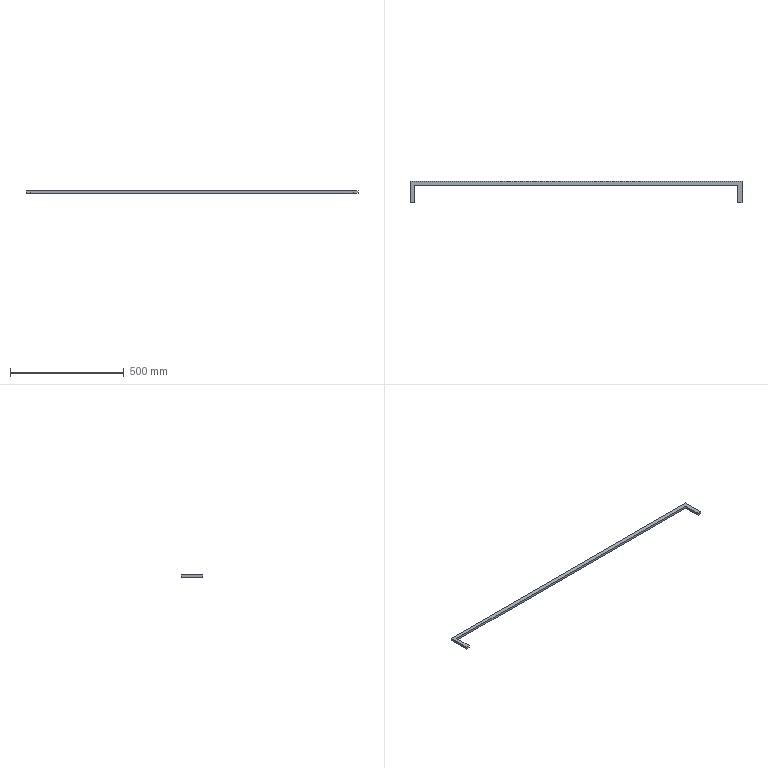Part | STEP file | 1 solid | 10 faces | box 1458 x 94 x 10 mm | volume 289800 mm3 | plane 10
STEP:
#1=CARTESIAN_POINT('',(0.,0.,0.));
#2=DIRECTION('',(0.,0.,1.));
#3=DIRECTION('',(1.,0.,0.));
#4=AXIS2_PLACEMENT_3D('',#1,#2,#3);
#5=CARTESIAN_POINT('',(-18.,0.,0.));
#6=VERTEX_POINT('',#5);
#7=CARTESIAN_POINT('',(-18.,94.,0.));
#8=VERTEX_POINT('',#7);
#9=CARTESIAN_POINT('',(-18.,0.,0.));
#10=DIRECTION('',(0.,1.,0.));
#11=VECTOR('',#10,1.);
#12=LINE('',#9,#11);
#13=CARTESIAN_POINT('',(1422.,0.,0.));
#14=DIRECTION('',(0.,0.,-1.));
#15=DIRECTION('',(-1.,0.,0.));
#16=AXIS2_PLACEMENT_3D('',#13,#14,#15);
#17=PLANE('',#16);
#18=CARTESIAN_POINT('',(1440.,0.));
#19=DIRECTION('',(0.,1.));
#20=VECTOR('',#19,1.);
#21=LINE('',#18,#20);
#22=(GEOMETRIC_REPRESENTATION_CONTEXT(2)PARAMETRIC_REPRESENTATION_CONTEXT()REPRESENTATION_CONTEXT('',''));
#23=DEFINITIONAL_REPRESENTATION('',(#21),#22);
#24=PCURVE('',#17,#23);
#25=CARTESIAN_POINT('',(-18.,0.,10.));
#26=DIRECTION('',(-1.,0.,0.));
#27=DIRECTION('',(0.,0.,1.));
#28=AXIS2_PLACEMENT_3D('',#25,#26,#27);
#29=PLANE('',#28);
#30=CARTESIAN_POINT('',(-10.,0.));
#31=DIRECTION('',(0.,1.));
#32=VECTOR('',#31,1.);
#33=LINE('',#30,#32);
#34=(GEOMETRIC_REPRESENTATION_CONTEXT(2)PARAMETRIC_REPRESENTATION_CONTEXT()REPRESENTATION_CONTEXT('',''));
#35=DEFINITIONAL_REPRESENTATION('',(#33),#34);
#36=PCURVE('',#29,#35);
#37=SURFACE_CURVE('',#12,(#24,#36),.PCURVE_S1.);
#38=EDGE_CURVE('',#6,#8,#37,.T.);
#39=ORIENTED_EDGE('',*,*,#38,.T.);
#40=CARTESIAN_POINT('',(1440.,94.,0.));
#41=VERTEX_POINT('',#40);
#42=CARTESIAN_POINT('',(1422.,94.,0.));
#43=DIRECTION('',(1.,0.,0.));
#44=VECTOR('',#43,1.);
#45=LINE('',#42,#44);
#46=CARTESIAN_POINT('',(0.,94.));
#47=DIRECTION('',(-1.,0.));
#48=VECTOR('',#47,1.);
#49=LINE('',#46,#48);
#50=(GEOMETRIC_REPRESENTATION_CONTEXT(2)PARAMETRIC_REPRESENTATION_CONTEXT()REPRESENTATION_CONTEXT('',''));
#51=DEFINITIONAL_REPRESENTATION('',(#49),#50);
#52=PCURVE('',#17,#51);
#53=CARTESIAN_POINT('',(0.,94.,10.));
#54=DIRECTION('',(0.,1.,0.));
#55=DIRECTION('',(0.,0.,1.));
#56=AXIS2_PLACEMENT_3D('',#53,#54,#55);
#57=PLANE('',#56);
#58=CARTESIAN_POINT('',(-10.,1422.));
#59=DIRECTION('',(0.,1.));
#60=VECTOR('',#59,1.);
#61=LINE('',#58,#60);
#62=(GEOMETRIC_REPRESENTATION_CONTEXT(2)PARAMETRIC_REPRESENTATION_CONTEXT()REPRESENTATION_CONTEXT('',''));
#63=DEFINITIONAL_REPRESENTATION('',(#61),#62);
#64=PCURVE('',#57,#63);
#65=SURFACE_CURVE('',#45,(#52,#64),.PCURVE_S1.);
#66=EDGE_CURVE('',#8,#41,#65,.T.);
#67=ORIENTED_EDGE('',*,*,#66,.T.);
#68=CARTESIAN_POINT('',(1440.,0.,0.));
#69=VERTEX_POINT('',#68);
#70=CARTESIAN_POINT('',(1440.,0.,0.));
#71=DIRECTION('',(0.,-1.,0.));
#72=VECTOR('',#71,1.);
#73=LINE('',#70,#72);
#74=CARTESIAN_POINT('',(-18.,0.));
#75=DIRECTION('',(0.,-1.));
#76=VECTOR('',#75,1.);
#77=LINE('',#74,#76);
#78=(GEOMETRIC_REPRESENTATION_CONTEXT(2)PARAMETRIC_REPRESENTATION_CONTEXT()REPRESENTATION_CONTEXT('',''));
#79=DEFINITIONAL_REPRESENTATION('',(#77),#78);
#80=PCURVE('',#17,#79);
#81=CARTESIAN_POINT('',(1440.,76.,10.));
#82=DIRECTION('',(1.,0.,0.));
#83=DIRECTION('',(0.,0.,-1.));
#84=AXIS2_PLACEMENT_3D('',#81,#82,#83);
#85=PLANE('',#84);
#86=CARTESIAN_POINT('',(10.,-76.));
#87=DIRECTION('',(0.,-1.));
#88=VECTOR('',#87,1.);
#89=LINE('',#86,#88);
#90=(GEOMETRIC_REPRESENTATION_CONTEXT(2)PARAMETRIC_REPRESENTATION_CONTEXT()REPRESENTATION_CONTEXT('',''));
#91=DEFINITIONAL_REPRESENTATION('',(#89),#90);
#92=PCURVE('',#85,#91);
#93=SURFACE_CURVE('',#73,(#80,#92),.PCURVE_S1.);
#94=EDGE_CURVE('',#41,#69,#93,.T.);
#95=ORIENTED_EDGE('',*,*,#94,.T.);
#96=CARTESIAN_POINT('',(1422.,0.,0.));
#97=VERTEX_POINT('',#96);
#98=CARTESIAN_POINT('',(1422.,0.,0.));
#99=DIRECTION('',(-1.,0.,0.));
#100=VECTOR('',#99,1.);
#101=LINE('',#98,#100);
#102=CARTESIAN_POINT('',(0.,0.));
#103=DIRECTION('',(1.,0.));
#104=VECTOR('',#103,1.);
#105=LINE('',#102,#104);
#106=(GEOMETRIC_REPRESENTATION_CONTEXT(2)PARAMETRIC_REPRESENTATION_CONTEXT()REPRESENTATION_CONTEXT('',''));
#107=DEFINITIONAL_REPRESENTATION('',(#105),#106);
#108=PCURVE('',#17,#107);
#109=CARTESIAN_POINT('',(1440.,0.,10.));
#110=DIRECTION('',(0.,-1.,0.));
#111=DIRECTION('',(0.,0.,-1.));
#112=AXIS2_PLACEMENT_3D('',#109,#110,#111);
#113=PLANE('',#112);
#114=CARTESIAN_POINT('',(10.,-18.));
#115=DIRECTION('',(0.,-1.));
#116=VECTOR('',#115,1.);
#117=LINE('',#114,#116);
#118=(GEOMETRIC_REPRESENTATION_CONTEXT(2)PARAMETRIC_REPRESENTATION_CONTEXT()REPRESENTATION_CONTEXT('',''));
#119=DEFINITIONAL_REPRESENTATION('',(#117),#118);
#120=PCURVE('',#113,#119);
#121=SURFACE_CURVE('',#101,(#108,#120),.PCURVE_S1.);
#122=EDGE_CURVE('',#69,#97,#121,.T.);
#123=ORIENTED_EDGE('',*,*,#122,.T.);
#124=CARTESIAN_POINT('',(1422.,76.,0.));
#125=VERTEX_POINT('',#124);
#126=CARTESIAN_POINT('',(1422.,0.,0.));
#127=DIRECTION('',(0.,1.,0.));
#128=VECTOR('',#127,1.);
#129=LINE('',#126,#128);
#130=CARTESIAN_POINT('',(0.,0.));
#131=DIRECTION('',(0.,1.));
#132=VECTOR('',#131,1.);
#133=LINE('',#130,#132);
#134=(GEOMETRIC_REPRESENTATION_CONTEXT(2)PARAMETRIC_REPRESENTATION_CONTEXT()REPRESENTATION_CONTEXT('',''));
#135=DEFINITIONAL_REPRESENTATION('',(#133),#134);
#136=PCURVE('',#17,#135);
#137=CARTESIAN_POINT('',(1422.,76.,10.));
#138=DIRECTION('',(1.,0.,0.));
#139=DIRECTION('',(0.,0.,-1.));
#140=AXIS2_PLACEMENT_3D('',#137,#138,#139);
#141=PLANE('',#140);
#142=CARTESIAN_POINT('',(10.,-76.));
#143=DIRECTION('',(0.,1.));
#144=VECTOR('',#143,1.);
#145=LINE('',#142,#144);
#146=(GEOMETRIC_REPRESENTATION_CONTEXT(2)PARAMETRIC_REPRESENTATION_CONTEXT()REPRESENTATION_CONTEXT('',''));
#147=DEFINITIONAL_REPRESENTATION('',(#145),#146);
#148=PCURVE('',#141,#147);
#149=SURFACE_CURVE('',#129,(#136,#148),.PCURVE_S1.);
#150=EDGE_CURVE('',#97,#125,#149,.T.);
#151=ORIENTED_EDGE('',*,*,#150,.T.);
#152=CARTESIAN_POINT('',(0.,76.,0.));
#153=VERTEX_POINT('',#152);
#154=CARTESIAN_POINT('',(1422.,76.,0.));
#155=DIRECTION('',(-1.,0.,0.));
#156=VECTOR('',#155,1.);
#157=LINE('',#154,#156);
#158=CARTESIAN_POINT('',(0.,76.));
#159=DIRECTION('',(1.,0.));
#160=VECTOR('',#159,1.);
#161=LINE('',#158,#160);
#162=(GEOMETRIC_REPRESENTATION_CONTEXT(2)PARAMETRIC_REPRESENTATION_CONTEXT()REPRESENTATION_CONTEXT('',''));
#163=DEFINITIONAL_REPRESENTATION('',(#161),#162);
#164=PCURVE('',#17,#163);
#165=CARTESIAN_POINT('',(0.,76.,10.));
#166=DIRECTION('',(0.,1.,0.));
#167=DIRECTION('',(0.,0.,1.));
#168=AXIS2_PLACEMENT_3D('',#165,#166,#167);
#169=PLANE('',#168);
#170=CARTESIAN_POINT('',(-10.,1422.));
#171=DIRECTION('',(0.,-1.));
#172=VECTOR('',#171,1.);
#173=LINE('',#170,#172);
#174=(GEOMETRIC_REPRESENTATION_CONTEXT(2)PARAMETRIC_REPRESENTATION_CONTEXT()REPRESENTATION_CONTEXT('',''));
#175=DEFINITIONAL_REPRESENTATION('',(#173),#174);
#176=PCURVE('',#169,#175);
#177=SURFACE_CURVE('',#157,(#164,#176),.PCURVE_S1.);
#178=EDGE_CURVE('',#125,#153,#177,.T.);
#179=ORIENTED_EDGE('',*,*,#178,.T.);
#180=CARTESIAN_POINT('',(0.,0.,0.));
#181=VERTEX_POINT('',#180);
#182=CARTESIAN_POINT('',(0.,0.,0.));
#183=DIRECTION('',(0.,-1.,0.));
#184=VECTOR('',#183,1.);
#185=LINE('',#182,#184);
#186=CARTESIAN_POINT('',(1422.,0.));
#187=DIRECTION('',(0.,-1.));
#188=VECTOR('',#187,1.);
#189=LINE('',#186,#188);
#190=(GEOMETRIC_REPRESENTATION_CONTEXT(2)PARAMETRIC_REPRESENTATION_CONTEXT()REPRESENTATION_CONTEXT('',''));
#191=DEFINITIONAL_REPRESENTATION('',(#189),#190);
#192=PCURVE('',#17,#191);
#193=CARTESIAN_POINT('',(0.,0.,10.));
#194=DIRECTION('',(-1.,0.,0.));
#195=DIRECTION('',(0.,0.,1.));
#196=AXIS2_PLACEMENT_3D('',#193,#194,#195);
#197=PLANE('',#196);
#198=CARTESIAN_POINT('',(-10.,0.));
#199=DIRECTION('',(0.,-1.));
#200=VECTOR('',#199,1.);
#201=LINE('',#198,#200);
#202=(GEOMETRIC_REPRESENTATION_CONTEXT(2)PARAMETRIC_REPRESENTATION_CONTEXT()REPRESENTATION_CONTEXT('',''));
#203=DEFINITIONAL_REPRESENTATION('',(#201),#202);
#204=PCURVE('',#197,#203);
#205=SURFACE_CURVE('',#185,(#192,#204),.PCURVE_S1.);
#206=EDGE_CURVE('',#153,#181,#205,.T.);
#207=ORIENTED_EDGE('',*,*,#206,.T.);
#208=CARTESIAN_POINT('',(1422.,0.,0.));
#209=DIRECTION('',(-1.,0.,0.));
#210=VECTOR('',#209,1.);
#211=LINE('',#208,#210);
#212=CARTESIAN_POINT('',(0.,0.));
#213=DIRECTION('',(1.,0.));
#214=VECTOR('',#213,1.);
#215=LINE('',#212,#214);
#216=(GEOMETRIC_REPRESENTATION_CONTEXT(2)PARAMETRIC_REPRESENTATION_CONTEXT()REPRESENTATION_CONTEXT('',''));
#217=DEFINITIONAL_REPRESENTATION('',(#215),#216);
#218=PCURVE('',#17,#217);
#219=CARTESIAN_POINT('',(0.,0.,10.));
#220=DIRECTION('',(0.,-1.,0.));
#221=DIRECTION('',(0.,0.,-1.));
#222=AXIS2_PLACEMENT_3D('',#219,#220,#221);
#223=PLANE('',#222);
#224=CARTESIAN_POINT('',(10.,1422.));
#225=DIRECTION('',(0.,-1.));
#226=VECTOR('',#225,1.);
#227=LINE('',#224,#226);
#228=(GEOMETRIC_REPRESENTATION_CONTEXT(2)PARAMETRIC_REPRESENTATION_CONTEXT()REPRESENTATION_CONTEXT('',''));
#229=DEFINITIONAL_REPRESENTATION('',(#227),#228);
#230=PCURVE('',#223,#229);
#231=SURFACE_CURVE('',#211,(#218,#230),.PCURVE_S1.);
#232=EDGE_CURVE('',#181,#6,#231,.T.);
#233=ORIENTED_EDGE('',*,*,#232,.T.);
#234=EDGE_LOOP('',(#39,#67,#95,#123,#151,#179,#207,#233));
#235=FACE_BOUND('',#234,.T.);
#236=ADVANCED_FACE('',(#235),#17,.T.);
#237=ORIENTED_EDGE('',*,*,#66,.F.);
#238=CARTESIAN_POINT('',(-18.,94.,10.));
#239=VERTEX_POINT('',#238);
#240=CARTESIAN_POINT('',(-18.,94.,10.));
#241=DIRECTION('',(0.,0.,1.));
#242=VECTOR('',#241,1.);
#243=LINE('',#240,#242);
#244=CARTESIAN_POINT('',(0.,-18.));
#245=DIRECTION('',(1.,0.));
#246=VECTOR('',#245,1.);
#247=LINE('',#244,#246);
#248=(GEOMETRIC_REPRESENTATION_CONTEXT(2)PARAMETRIC_REPRESENTATION_CONTEXT()REPRESENTATION_CONTEXT('',''));
#249=DEFINITIONAL_REPRESENTATION('',(#247),#248);
#250=PCURVE('',#57,#249);
#251=CARTESIAN_POINT('',(0.,94.));
#252=DIRECTION('',(1.,0.));
#253=VECTOR('',#252,1.);
#254=LINE('',#251,#253);
#255=(GEOMETRIC_REPRESENTATION_CONTEXT(2)PARAMETRIC_REPRESENTATION_CONTEXT()REPRESENTATION_CONTEXT('',''));
#256=DEFINITIONAL_REPRESENTATION('',(#254),#255);
#257=PCURVE('',#29,#256);
#258=SURFACE_CURVE('',#243,(#250,#257),.PCURVE_S1.);
#259=EDGE_CURVE('',#8,#239,#258,.T.);
#260=ORIENTED_EDGE('',*,*,#259,.T.);
#261=CARTESIAN_POINT('',(1440.,94.,10.));
#262=VERTEX_POINT('',#261);
#263=CARTESIAN_POINT('',(0.,94.,10.));
#264=DIRECTION('',(1.,0.,0.));
#265=VECTOR('',#264,1.);
#266=LINE('',#263,#265);
#267=CARTESIAN_POINT('',(0.,0.));
#268=DIRECTION('',(0.,1.));
#269=VECTOR('',#268,1.);
#270=LINE('',#267,#269);
#271=(GEOMETRIC_REPRESENTATION_CONTEXT(2)PARAMETRIC_REPRESENTATION_CONTEXT()REPRESENTATION_CONTEXT('',''));
#272=DEFINITIONAL_REPRESENTATION('',(#270),#271);
#273=PCURVE('',#57,#272);
#274=CARTESIAN_POINT('',(1422.,0.,10.));
#275=DIRECTION('',(0.,0.,-1.));
#276=DIRECTION('',(-1.,0.,0.));
#277=AXIS2_PLACEMENT_3D('',#274,#275,#276);
#278=PLANE('',#277);
#279=CARTESIAN_POINT('',(1422.,94.));
#280=DIRECTION('',(-1.,0.));
#281=VECTOR('',#280,1.);
#282=LINE('',#279,#281);
#283=(GEOMETRIC_REPRESENTATION_CONTEXT(2)PARAMETRIC_REPRESENTATION_CONTEXT()REPRESENTATION_CONTEXT('',''));
#284=DEFINITIONAL_REPRESENTATION('',(#282),#283);
#285=PCURVE('',#278,#284);
#286=SURFACE_CURVE('',#266,(#273,#285),.PCURVE_S1.);
#287=EDGE_CURVE('',#239,#262,#286,.T.);
#288=ORIENTED_EDGE('',*,*,#287,.T.);
#289=CARTESIAN_POINT('',(1440.,94.,10.));
#290=DIRECTION('',(0.,0.,-1.));
#291=VECTOR('',#290,1.);
#292=LINE('',#289,#291);
#293=CARTESIAN_POINT('',(0.,1440.));
#294=DIRECTION('',(-1.,0.));
#295=VECTOR('',#294,1.);
#296=LINE('',#293,#295);
#297=(GEOMETRIC_REPRESENTATION_CONTEXT(2)PARAMETRIC_REPRESENTATION_CONTEXT()REPRESENTATION_CONTEXT('',''));
#298=DEFINITIONAL_REPRESENTATION('',(#296),#297);
#299=PCURVE('',#57,#298);
#300=CARTESIAN_POINT('',(0.,18.));
#301=DIRECTION('',(1.,0.));
#302=VECTOR('',#301,1.);
#303=LINE('',#300,#302);
#304=(GEOMETRIC_REPRESENTATION_CONTEXT(2)PARAMETRIC_REPRESENTATION_CONTEXT()REPRESENTATION_CONTEXT('',''));
#305=DEFINITIONAL_REPRESENTATION('',(#303),#304);
#306=PCURVE('',#85,#305);
#307=SURFACE_CURVE('',#292,(#299,#306),.PCURVE_S1.);
#308=EDGE_CURVE('',#262,#41,#307,.T.);
#309=ORIENTED_EDGE('',*,*,#308,.T.);
#310=EDGE_LOOP('',(#237,#260,#288,#309));
#311=FACE_BOUND('',#310,.T.);
#312=ADVANCED_FACE('',(#311),#57,.T.);
#313=ORIENTED_EDGE('',*,*,#38,.F.);
#314=CARTESIAN_POINT('',(-18.,0.,10.));
#315=VERTEX_POINT('',#314);
#316=CARTESIAN_POINT('',(-18.,0.,10.));
#317=DIRECTION('',(0.,0.,1.));
#318=VECTOR('',#317,1.);
#319=LINE('',#316,#318);
#320=CARTESIAN_POINT('',(0.,0.));
#321=DIRECTION('',(1.,0.));
#322=VECTOR('',#321,1.);
#323=LINE('',#320,#322);
#324=(GEOMETRIC_REPRESENTATION_CONTEXT(2)PARAMETRIC_REPRESENTATION_CONTEXT()REPRESENTATION_CONTEXT('',''));
#325=DEFINITIONAL_REPRESENTATION('',(#323),#324);
#326=PCURVE('',#29,#325);
#327=CARTESIAN_POINT('',(0.,-18.));
#328=DIRECTION('',(-1.,0.));
#329=VECTOR('',#328,1.);
#330=LINE('',#327,#329);
#331=(GEOMETRIC_REPRESENTATION_CONTEXT(2)PARAMETRIC_REPRESENTATION_CONTEXT()REPRESENTATION_CONTEXT('',''));
#332=DEFINITIONAL_REPRESENTATION('',(#330),#331);
#333=PCURVE('',#223,#332);
#334=SURFACE_CURVE('',#319,(#326,#333),.PCURVE_S1.);
#335=EDGE_CURVE('',#6,#315,#334,.T.);
#336=ORIENTED_EDGE('',*,*,#335,.T.);
#337=CARTESIAN_POINT('',(-18.,0.,10.));
#338=DIRECTION('',(0.,1.,0.));
#339=VECTOR('',#338,1.);
#340=LINE('',#337,#339);
#341=CARTESIAN_POINT('',(0.,0.));
#342=DIRECTION('',(0.,1.));
#343=VECTOR('',#342,1.);
#344=LINE('',#341,#343);
#345=(GEOMETRIC_REPRESENTATION_CONTEXT(2)PARAMETRIC_REPRESENTATION_CONTEXT()REPRESENTATION_CONTEXT('',''));
#346=DEFINITIONAL_REPRESENTATION('',(#344),#345);
#347=PCURVE('',#29,#346);
#348=CARTESIAN_POINT('',(1440.,0.));
#349=DIRECTION('',(0.,1.));
#350=VECTOR('',#349,1.);
#351=LINE('',#348,#350);
#352=(GEOMETRIC_REPRESENTATION_CONTEXT(2)PARAMETRIC_REPRESENTATION_CONTEXT()REPRESENTATION_CONTEXT('',''));
#353=DEFINITIONAL_REPRESENTATION('',(#351),#352);
#354=PCURVE('',#278,#353);
#355=SURFACE_CURVE('',#340,(#347,#354),.PCURVE_S1.);
#356=EDGE_CURVE('',#315,#239,#355,.T.);
#357=ORIENTED_EDGE('',*,*,#356,.T.);
#358=ORIENTED_EDGE('',*,*,#259,.F.);
#359=EDGE_LOOP('',(#313,#336,#357,#358));
#360=FACE_BOUND('',#359,.T.);
#361=ADVANCED_FACE('',(#360),#29,.T.);
#362=ORIENTED_EDGE('',*,*,#232,.F.);
#363=CARTESIAN_POINT('',(0.,0.,10.));
#364=VERTEX_POINT('',#363);
#365=CARTESIAN_POINT('',(0.,0.,10.));
#366=DIRECTION('',(0.,0.,1.));
#367=VECTOR('',#366,1.);
#368=LINE('',#365,#367);
#369=CARTESIAN_POINT('',(0.,0.));
#370=DIRECTION('',(-1.,0.));
#371=VECTOR('',#370,1.);
#372=LINE('',#369,#371);
#373=(GEOMETRIC_REPRESENTATION_CONTEXT(2)PARAMETRIC_REPRESENTATION_CONTEXT()REPRESENTATION_CONTEXT('',''));
#374=DEFINITIONAL_REPRESENTATION('',(#372),#373);
#375=PCURVE('',#223,#374);
#376=CARTESIAN_POINT('',(0.,0.));
#377=DIRECTION('',(1.,0.));
#378=VECTOR('',#377,1.);
#379=LINE('',#376,#378);
#380=(GEOMETRIC_REPRESENTATION_CONTEXT(2)PARAMETRIC_REPRESENTATION_CONTEXT()REPRESENTATION_CONTEXT('',''));
#381=DEFINITIONAL_REPRESENTATION('',(#379),#380);
#382=PCURVE('',#197,#381);
#383=SURFACE_CURVE('',#368,(#375,#382),.PCURVE_S1.);
#384=EDGE_CURVE('',#181,#364,#383,.T.);
#385=ORIENTED_EDGE('',*,*,#384,.T.);
#386=CARTESIAN_POINT('',(0.,0.,10.));
#387=DIRECTION('',(-1.,0.,0.));
#388=VECTOR('',#387,1.);
#389=LINE('',#386,#388);
#390=CARTESIAN_POINT('',(0.,0.));
#391=DIRECTION('',(0.,-1.));
#392=VECTOR('',#391,1.);
#393=LINE('',#390,#392);
#394=(GEOMETRIC_REPRESENTATION_CONTEXT(2)PARAMETRIC_REPRESENTATION_CONTEXT()REPRESENTATION_CONTEXT('',''));
#395=DEFINITIONAL_REPRESENTATION('',(#393),#394);
#396=PCURVE('',#223,#395);
#397=CARTESIAN_POINT('',(1422.,0.));
#398=DIRECTION('',(1.,0.));
#399=VECTOR('',#398,1.);
#400=LINE('',#397,#399);
#401=(GEOMETRIC_REPRESENTATION_CONTEXT(2)PARAMETRIC_REPRESENTATION_CONTEXT()REPRESENTATION_CONTEXT('',''));
#402=DEFINITIONAL_REPRESENTATION('',(#400),#401);
#403=PCURVE('',#278,#402);
#404=SURFACE_CURVE('',#389,(#396,#403),.PCURVE_S1.);
#405=EDGE_CURVE('',#364,#315,#404,.T.);
#406=ORIENTED_EDGE('',*,*,#405,.T.);
#407=ORIENTED_EDGE('',*,*,#335,.F.);
#408=EDGE_LOOP('',(#362,#385,#406,#407));
#409=FACE_BOUND('',#408,.T.);
#410=ADVANCED_FACE('',(#409),#223,.T.);
#411=CARTESIAN_POINT('',(0.,76.,10.));
#412=VERTEX_POINT('',#411);
#413=CARTESIAN_POINT('',(0.,0.,10.));
#414=DIRECTION('',(0.,1.,0.));
#415=VECTOR('',#414,1.);
#416=LINE('',#413,#415);
#417=CARTESIAN_POINT('',(0.,0.));
#418=DIRECTION('',(0.,1.));
#419=VECTOR('',#418,1.);
#420=LINE('',#417,#419);
#421=(GEOMETRIC_REPRESENTATION_CONTEXT(2)PARAMETRIC_REPRESENTATION_CONTEXT()REPRESENTATION_CONTEXT('',''));
#422=DEFINITIONAL_REPRESENTATION('',(#420),#421);
#423=PCURVE('',#197,#422);
#424=CARTESIAN_POINT('',(1422.,0.));
#425=DIRECTION('',(0.,1.));
#426=VECTOR('',#425,1.);
#427=LINE('',#424,#426);
#428=(GEOMETRIC_REPRESENTATION_CONTEXT(2)PARAMETRIC_REPRESENTATION_CONTEXT()REPRESENTATION_CONTEXT('',''));
#429=DEFINITIONAL_REPRESENTATION('',(#427),#428);
#430=PCURVE('',#278,#429);
#431=SURFACE_CURVE('',#416,(#423,#430),.PCURVE_S1.);
#432=EDGE_CURVE('',#364,#412,#431,.T.);
#433=ORIENTED_EDGE('',*,*,#432,.F.);
#434=ORIENTED_EDGE('',*,*,#384,.F.);
#435=ORIENTED_EDGE('',*,*,#206,.F.);
#436=CARTESIAN_POINT('',(0.,76.,10.));
#437=DIRECTION('',(0.,0.,-1.));
#438=VECTOR('',#437,1.);
#439=LINE('',#436,#438);
#440=CARTESIAN_POINT('',(0.,76.));
#441=DIRECTION('',(-1.,0.));
#442=VECTOR('',#441,1.);
#443=LINE('',#440,#442);
#444=(GEOMETRIC_REPRESENTATION_CONTEXT(2)PARAMETRIC_REPRESENTATION_CONTEXT()REPRESENTATION_CONTEXT('',''));
#445=DEFINITIONAL_REPRESENTATION('',(#443),#444);
#446=PCURVE('',#197,#445);
#447=CARTESIAN_POINT('',(0.,0.));
#448=DIRECTION('',(-1.,0.));
#449=VECTOR('',#448,1.);
#450=LINE('',#447,#449);
#451=(GEOMETRIC_REPRESENTATION_CONTEXT(2)PARAMETRIC_REPRESENTATION_CONTEXT()REPRESENTATION_CONTEXT('',''));
#452=DEFINITIONAL_REPRESENTATION('',(#450),#451);
#453=PCURVE('',#169,#452);
#454=SURFACE_CURVE('',#439,(#446,#453),.PCURVE_S1.);
#455=EDGE_CURVE('',#412,#153,#454,.T.);
#456=ORIENTED_EDGE('',*,*,#455,.F.);
#457=EDGE_LOOP('',(#433,#434,#435,#456));
#458=FACE_BOUND('',#457,.T.);
#459=ADVANCED_FACE('',(#458),#197,.F.);
#460=CARTESIAN_POINT('',(1422.,76.,10.));
#461=VERTEX_POINT('',#460);
#462=CARTESIAN_POINT('',(0.,76.,10.));
#463=DIRECTION('',(1.,0.,0.));
#464=VECTOR('',#463,1.);
#465=LINE('',#462,#464);
#466=CARTESIAN_POINT('',(0.,0.));
#467=DIRECTION('',(0.,1.));
#468=VECTOR('',#467,1.);
#469=LINE('',#466,#468);
#470=(GEOMETRIC_REPRESENTATION_CONTEXT(2)PARAMETRIC_REPRESENTATION_CONTEXT()REPRESENTATION_CONTEXT('',''));
#471=DEFINITIONAL_REPRESENTATION('',(#469),#470);
#472=PCURVE('',#169,#471);
#473=CARTESIAN_POINT('',(1422.,76.));
#474=DIRECTION('',(-1.,0.));
#475=VECTOR('',#474,1.);
#476=LINE('',#473,#475);
#477=(GEOMETRIC_REPRESENTATION_CONTEXT(2)PARAMETRIC_REPRESENTATION_CONTEXT()REPRESENTATION_CONTEXT('',''));
#478=DEFINITIONAL_REPRESENTATION('',(#476),#477);
#479=PCURVE('',#278,#478);
#480=SURFACE_CURVE('',#465,(#472,#479),.PCURVE_S1.);
#481=EDGE_CURVE('',#412,#461,#480,.T.);
#482=ORIENTED_EDGE('',*,*,#481,.F.);
#483=ORIENTED_EDGE('',*,*,#455,.T.);
#484=ORIENTED_EDGE('',*,*,#178,.F.);
#485=CARTESIAN_POINT('',(1422.,76.,10.));
#486=DIRECTION('',(0.,0.,-1.));
#487=VECTOR('',#486,1.);
#488=LINE('',#485,#487);
#489=CARTESIAN_POINT('',(0.,1422.));
#490=DIRECTION('',(-1.,0.));
#491=VECTOR('',#490,1.);
#492=LINE('',#489,#491);
#493=(GEOMETRIC_REPRESENTATION_CONTEXT(2)PARAMETRIC_REPRESENTATION_CONTEXT()REPRESENTATION_CONTEXT('',''));
#494=DEFINITIONAL_REPRESENTATION('',(#492),#493);
#495=PCURVE('',#169,#494);
#496=CARTESIAN_POINT('',(0.,0.));
#497=DIRECTION('',(1.,0.));
#498=VECTOR('',#497,1.);
#499=LINE('',#496,#498);
#500=(GEOMETRIC_REPRESENTATION_CONTEXT(2)PARAMETRIC_REPRESENTATION_CONTEXT()REPRESENTATION_CONTEXT('',''));
#501=DEFINITIONAL_REPRESENTATION('',(#499),#500);
#502=PCURVE('',#141,#501);
#503=SURFACE_CURVE('',#488,(#495,#502),.PCURVE_S1.);
#504=EDGE_CURVE('',#461,#125,#503,.T.);
#505=ORIENTED_EDGE('',*,*,#504,.F.);
#506=EDGE_LOOP('',(#482,#483,#484,#505));
#507=FACE_BOUND('',#506,.T.);
#508=ADVANCED_FACE('',(#507),#169,.F.);
#509=CARTESIAN_POINT('',(1422.,0.,10.));
#510=VERTEX_POINT('',#509);
#511=CARTESIAN_POINT('',(1422.,76.,10.));
#512=DIRECTION('',(0.,-1.,0.));
#513=VECTOR('',#512,1.);
#514=LINE('',#511,#513);
#515=CARTESIAN_POINT('',(0.,0.));
#516=DIRECTION('',(0.,-1.));
#517=VECTOR('',#516,1.);
#518=LINE('',#515,#517);
#519=(GEOMETRIC_REPRESENTATION_CONTEXT(2)PARAMETRIC_REPRESENTATION_CONTEXT()REPRESENTATION_CONTEXT('',''));
#520=DEFINITIONAL_REPRESENTATION('',(#518),#519);
#521=PCURVE('',#141,#520);
#522=CARTESIAN_POINT('',(0.,76.));
#523=DIRECTION('',(0.,-1.));
#524=VECTOR('',#523,1.);
#525=LINE('',#522,#524);
#526=(GEOMETRIC_REPRESENTATION_CONTEXT(2)PARAMETRIC_REPRESENTATION_CONTEXT()REPRESENTATION_CONTEXT('',''));
#527=DEFINITIONAL_REPRESENTATION('',(#525),#526);
#528=PCURVE('',#278,#527);
#529=SURFACE_CURVE('',#514,(#521,#528),.PCURVE_S1.);
#530=EDGE_CURVE('',#461,#510,#529,.T.);
#531=ORIENTED_EDGE('',*,*,#530,.F.);
#532=ORIENTED_EDGE('',*,*,#504,.T.);
#533=ORIENTED_EDGE('',*,*,#150,.F.);
#534=CARTESIAN_POINT('',(1422.,0.,10.));
#535=DIRECTION('',(0.,0.,-1.));
#536=VECTOR('',#535,1.);
#537=LINE('',#534,#536);
#538=CARTESIAN_POINT('',(0.,-76.));
#539=DIRECTION('',(1.,0.));
#540=VECTOR('',#539,1.);
#541=LINE('',#538,#540);
#542=(GEOMETRIC_REPRESENTATION_CONTEXT(2)PARAMETRIC_REPRESENTATION_CONTEXT()REPRESENTATION_CONTEXT('',''));
#543=DEFINITIONAL_REPRESENTATION('',(#541),#542);
#544=PCURVE('',#141,#543);
#545=CARTESIAN_POINT('',(0.,-18.));
#546=DIRECTION('',(1.,0.));
#547=VECTOR('',#546,1.);
#548=LINE('',#545,#547);
#549=(GEOMETRIC_REPRESENTATION_CONTEXT(2)PARAMETRIC_REPRESENTATION_CONTEXT()REPRESENTATION_CONTEXT('',''));
#550=DEFINITIONAL_REPRESENTATION('',(#548),#549);
#551=PCURVE('',#113,#550);
#552=SURFACE_CURVE('',#537,(#544,#551),.PCURVE_S1.);
#553=EDGE_CURVE('',#510,#97,#552,.T.);
#554=ORIENTED_EDGE('',*,*,#553,.F.);
#555=EDGE_LOOP('',(#531,#532,#533,#554));
#556=FACE_BOUND('',#555,.T.);
#557=ADVANCED_FACE('',(#556),#141,.F.);
#558=ORIENTED_EDGE('',*,*,#122,.F.);
#559=CARTESIAN_POINT('',(1440.,0.,10.));
#560=VERTEX_POINT('',#559);
#561=CARTESIAN_POINT('',(1440.,0.,10.));
#562=DIRECTION('',(0.,0.,1.));
#563=VECTOR('',#562,1.);
#564=LINE('',#561,#563);
#565=CARTESIAN_POINT('',(0.,0.));
#566=DIRECTION('',(-1.,0.));
#567=VECTOR('',#566,1.);
#568=LINE('',#565,#567);
#569=(GEOMETRIC_REPRESENTATION_CONTEXT(2)PARAMETRIC_REPRESENTATION_CONTEXT()REPRESENTATION_CONTEXT('',''));
#570=DEFINITIONAL_REPRESENTATION('',(#568),#569);
#571=PCURVE('',#113,#570);
#572=CARTESIAN_POINT('',(0.,-76.));
#573=DIRECTION('',(-1.,0.));
#574=VECTOR('',#573,1.);
#575=LINE('',#572,#574);
#576=(GEOMETRIC_REPRESENTATION_CONTEXT(2)PARAMETRIC_REPRESENTATION_CONTEXT()REPRESENTATION_CONTEXT('',''));
#577=DEFINITIONAL_REPRESENTATION('',(#575),#576);
#578=PCURVE('',#85,#577);
#579=SURFACE_CURVE('',#564,(#571,#578),.PCURVE_S1.);
#580=EDGE_CURVE('',#69,#560,#579,.T.);
#581=ORIENTED_EDGE('',*,*,#580,.T.);
#582=CARTESIAN_POINT('',(1440.,0.,10.));
#583=DIRECTION('',(-1.,0.,0.));
#584=VECTOR('',#583,1.);
#585=LINE('',#582,#584);
#586=CARTESIAN_POINT('',(0.,0.));
#587=DIRECTION('',(0.,-1.));
#588=VECTOR('',#587,1.);
#589=LINE('',#586,#588);
#590=(GEOMETRIC_REPRESENTATION_CONTEXT(2)PARAMETRIC_REPRESENTATION_CONTEXT()REPRESENTATION_CONTEXT('',''));
#591=DEFINITIONAL_REPRESENTATION('',(#589),#590);
#592=PCURVE('',#113,#591);
#593=CARTESIAN_POINT('',(-18.,0.));
#594=DIRECTION('',(1.,0.));
#595=VECTOR('',#594,1.);
#596=LINE('',#593,#595);
#597=(GEOMETRIC_REPRESENTATION_CONTEXT(2)PARAMETRIC_REPRESENTATION_CONTEXT()REPRESENTATION_CONTEXT('',''));
#598=DEFINITIONAL_REPRESENTATION('',(#596),#597);
#599=PCURVE('',#278,#598);
#600=SURFACE_CURVE('',#585,(#592,#599),.PCURVE_S1.);
#601=EDGE_CURVE('',#560,#510,#600,.T.);
#602=ORIENTED_EDGE('',*,*,#601,.T.);
#603=ORIENTED_EDGE('',*,*,#553,.T.);
#604=EDGE_LOOP('',(#558,#581,#602,#603));
#605=FACE_BOUND('',#604,.T.);
#606=ADVANCED_FACE('',(#605),#113,.T.);
#607=ORIENTED_EDGE('',*,*,#94,.F.);
#608=ORIENTED_EDGE('',*,*,#308,.F.);
#609=CARTESIAN_POINT('',(1440.,76.,10.));
#610=DIRECTION('',(0.,-1.,0.));
#611=VECTOR('',#610,1.);
#612=LINE('',#609,#611);
#613=CARTESIAN_POINT('',(0.,0.));
#614=DIRECTION('',(0.,-1.));
#615=VECTOR('',#614,1.);
#616=LINE('',#613,#615);
#617=(GEOMETRIC_REPRESENTATION_CONTEXT(2)PARAMETRIC_REPRESENTATION_CONTEXT()REPRESENTATION_CONTEXT('',''));
#618=DEFINITIONAL_REPRESENTATION('',(#616),#617);
#619=PCURVE('',#85,#618);
#620=CARTESIAN_POINT('',(-18.,76.));
#621=DIRECTION('',(0.,-1.));
#622=VECTOR('',#621,1.);
#623=LINE('',#620,#622);
#624=(GEOMETRIC_REPRESENTATION_CONTEXT(2)PARAMETRIC_REPRESENTATION_CONTEXT()REPRESENTATION_CONTEXT('',''));
#625=DEFINITIONAL_REPRESENTATION('',(#623),#624);
#626=PCURVE('',#278,#625);
#627=SURFACE_CURVE('',#612,(#619,#626),.PCURVE_S1.);
#628=EDGE_CURVE('',#262,#560,#627,.T.);
#629=ORIENTED_EDGE('',*,*,#628,.T.);
#630=ORIENTED_EDGE('',*,*,#580,.F.);
#631=EDGE_LOOP('',(#607,#608,#629,#630));
#632=FACE_BOUND('',#631,.T.);
#633=ADVANCED_FACE('',(#632),#85,.T.);
#634=ORIENTED_EDGE('',*,*,#628,.F.);
#635=ORIENTED_EDGE('',*,*,#287,.F.);
#636=ORIENTED_EDGE('',*,*,#356,.F.);
#637=ORIENTED_EDGE('',*,*,#405,.F.);
#638=ORIENTED_EDGE('',*,*,#432,.T.);
#639=ORIENTED_EDGE('',*,*,#481,.T.);
#640=ORIENTED_EDGE('',*,*,#530,.T.);
#641=ORIENTED_EDGE('',*,*,#601,.F.);
#642=EDGE_LOOP('',(#634,#635,#636,#637,#638,#639,#640,#641));
#643=FACE_BOUND('',#642,.T.);
#644=ADVANCED_FACE('',(#643),#278,.F.);
#645=CLOSED_SHELL('',(#236,#312,#361,#410,#459,#508,#557,#606,#633,#644));
#646=MANIFOLD_SOLID_BREP('',#645);
#647=(LENGTH_UNIT()NAMED_UNIT(*)SI_UNIT(.MILLI.,.METRE.));
#648=UNCERTAINTY_MEASURE_WITH_UNIT(LENGTH_MEASURE(0.0000001),#647,'','');
#649=(NAMED_UNIT(*)PLANE_ANGLE_UNIT()SI_UNIT($,.RADIAN.));
#650=(NAMED_UNIT(*)SI_UNIT($,.STERADIAN.)SOLID_ANGLE_UNIT());
#651=(GEOMETRIC_REPRESENTATION_CONTEXT(3)GLOBAL_UNCERTAINTY_ASSIGNED_CONTEXT((#648))GLOBAL_UNIT_ASSIGNED_CONTEXT((#647,#649,#650))REPRESENTATION_CONTEXT('',''));
#652=ADVANCED_BREP_SHAPE_REPRESENTATION('',(#4,#646),#651);